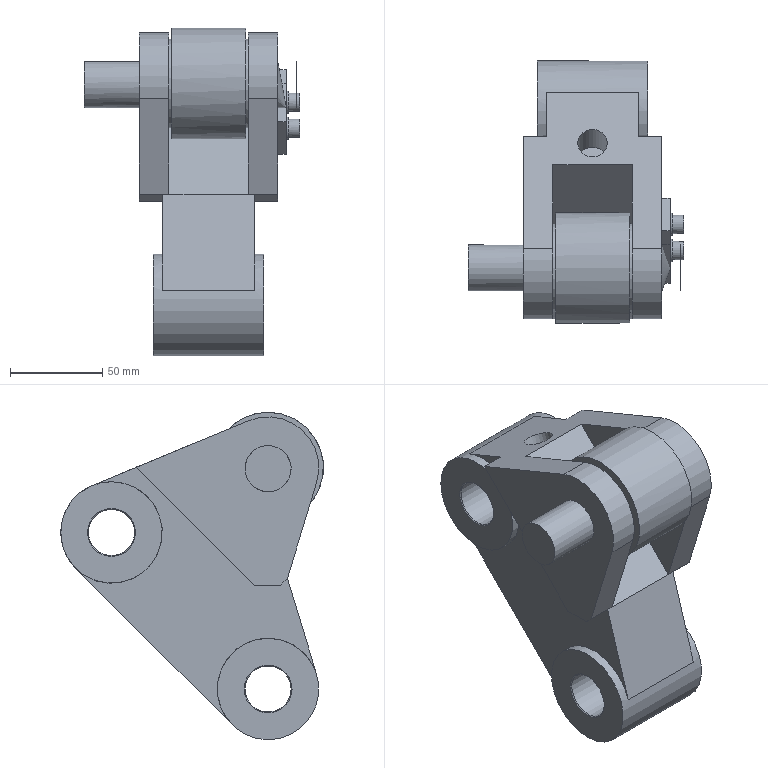Part | NX | features solid 2 | 2 solids | 62 faces | box 117 x 142.353 x 177.5 mm | volume 872934 mm3 | plane 37 | cylinder 17 | cone 8 | commonest cylinder face diameters 25 x5 55 x4 10 x2 12.2 x2 48 x2 16 x1